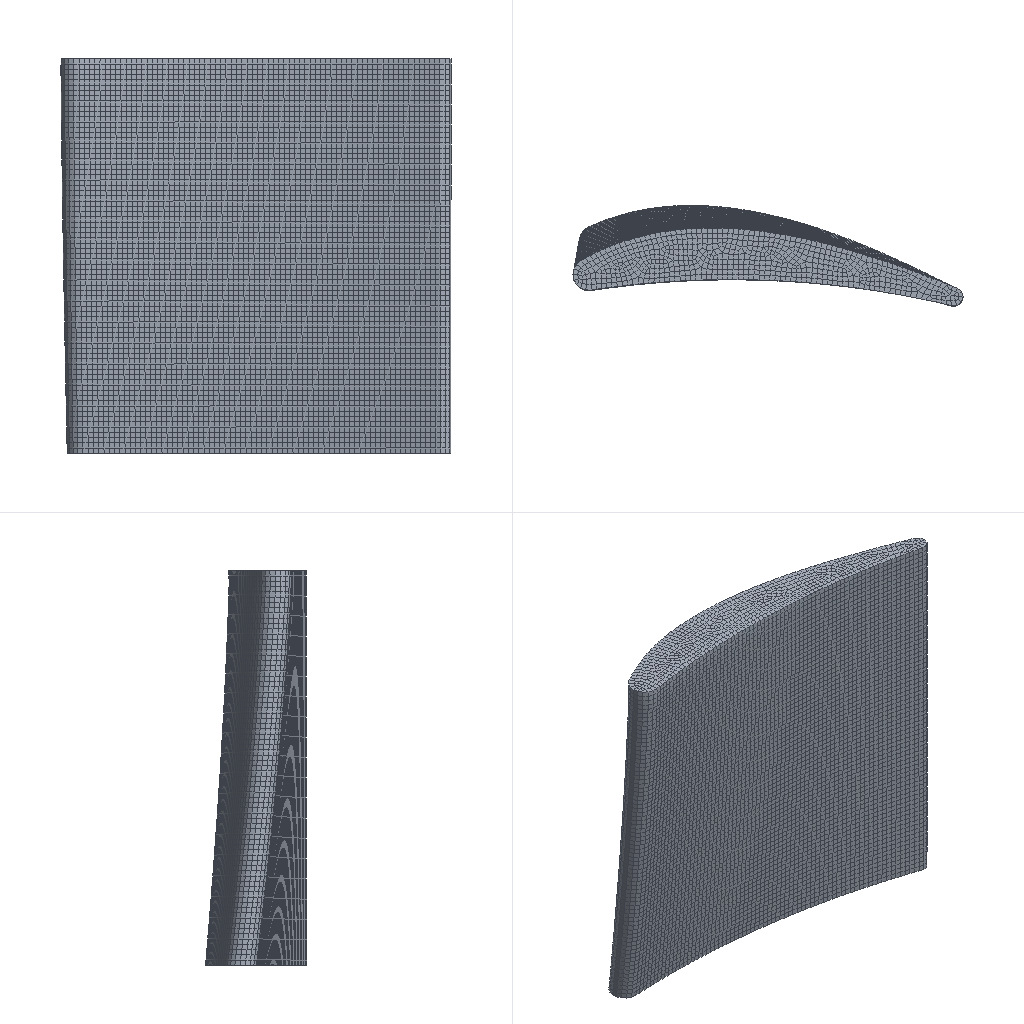Simulation study | abaqus
Set-up summary:
category,name,step,type,value,unit,region
solver,abaqus
solver,version,,,Abaqus/Explicit 2020
units,not stated in the deck,,not stated
analysis,deck,,transient,transient
load_step,Step-1,Step-1,transient
load_step,requested,,,1
mesh,nodes,,,58257
mesh,elements,,,54278
element_type,R3D3,,rigid,5378
element_type,C3D8R,,solid,48900
load,load commands in deck,,count,3
bc,support commands in deck,,count,7
material,MATERIAL-1,,in results
check,setup vs results,,match,"per instance, exact: element labels, types and connectivity; labels of the nodes the elements use; coordinates of those nodes at SINGLE_PRECISION in 2 of 2 instance(s)"
Abaqus input file, long lists of numbers shortened:
*Heading
** Job name: Job-1 Model name: Model-1
** Generated by: Abaqus/CAE 2020
*Preprint, echo=NO, model=NO, history=NO, contact=NO
**
** PARTS
**
*Part, name=tool-4
*Node
      1,           9.,           0.,         -90.
      2,          -9.,           0.,         -90.
** (2698 more lines like these left out)
*Element, type=R3D3
 1,   1, 149,   4
 2, 149, 178,   4
** (5376 more lines like these left out)
*Node
   2701,           0., -5.5109107e-16,         -90.
*Nset, nset=tool-4-RefPt_, internal
2701,
*Elset, elset=tool-4, generate
    1,  5378,     1
*End Part
**
*Part, name=work
*Node
      1,   43.691,  -25.705,         300.
      2,   39.949,  -24.243,         300.
** (55554 more lines like these left out)
*Element, type=C3D8R
    1,   667,   178,    32,   666,  1398,   909,   763,  1397
    2,   666,    32,    77,   431,  1397,   763,   808,  1162
** (48898 more lines like these left out)
*Nset, nset=Set-1, generate
     1,  55556,      1
*Elset, elset=Set-1, generate
     1,  48900,      1
** Section: Section-1
*Solid Section, elset=Set-1, material=Material-1
,
*End Part
**
**
** ASSEMBLY
**
*Assembly, name=Assembly
**
*Instance, name=tool-4-1, part=tool-4
  -45.177, 26.094, 89.811
  -45.177, 26.094, 89.811, -44.177, 26.094, 89.811, 5.
*End Instance
**
*Instance, name=work-1, part=work
   19.936,    15.042,        -100.
*End Instance
**
*Nset, nset=Set-1, instance=work-1, generate
   1,  731,    1
*Elset, elset=Set-1, instance=work-1, generate
   1,  652,    1
*Nset, nset=Set-2, instance=tool-4-1
 2701,
*Nset, nset=s_Set-3, instance=work-1, generate
     1,  55556,      1
*Elset, elset=s_Set-3, instance=work-1, generate
     1,  48900,      1
*Elset, elset=_m_Surf-1_SPOS, internal, instance=tool-4-1, generate
    1,  5378,     1
*Surface, type=ELEMENT, name=m_Surf-1
_m_Surf-1_SPOS, SPOS
*Surface, type=NODE, name=s_Set-3_CNS_, internal
s_Set-3, 1.
*Rigid Body, ref node=tool-4-1.tool-4-RefPt_, elset=tool-4-1.tool-4
*End Assembly
**
** MATERIALS
**
*Material, name=Material-1
*Damage Initiation, criterion=SHEAR
 0.1,0.,0.
*Damage Evolution, type=DISPLACEMENT
 1e-05,
*Density
 4.7e-09,
*Elastic
 1.2e+08, 0.28
*Plastic
800.,0.
**
** INTERACTION PROPERTIES
**
*Surface Interaction, name=IntProp-1
*Friction
 0.2,
*Surface Behavior, pressure-overclosure=HARD
** ----------------------------------------------------------------
**
** STEP: Step-1
**
*Step, name=Step-1, nlgeom=YES
*Dynamic, Explicit
, 0.08
*Bulk Viscosity
0.06, 1.2
** Mass Scaling: Semi-Automatic
**               Whole Model
*Fixed Mass Scaling, factor=5000.
**
** BOUNDARY CONDITIONS
**
** Name: BC-1 Type: 对称/反对称/完全固定
*Boundary
Set-1, ENCASTRE
** Name: [REDACTED] : Speed/Angular velocity
*Boundary, type=VELOCITY
Set-2, 1, 1, 2000.
Set-2, 2, 2, -2000.
Set-2, 3, 3
Set-2, 4, 4
Set-2, 5, 5
Set-2, 6, 6, 314.
**
** INTERACTIONS
**
** Interaction: Int-1
*Contact Pair, interaction=IntProp-1, mechanical constraint=KINEMATIC, cpset=Int-1
m_Surf-1, s_Set-3_CNS_
**
** OUTPUT REQUESTS
**
*Restart, write, number interval=1, time marks=NO
**
** FIELD OUTPUT: F-Output-1
**
*Output, field, number interval=50
*Node Output
A, CF, RF, RM, RT, U, V
*Element Output, directions=YES
E, EVF, LE, MISES, MISESMAX, PE, PEEQ, PEEQVAVG, PEVAVG, S, STATUS, SVAVG, YIELDPOT
*Contact Output
CSTRESS,
**
** HISTORY OUTPUT: H-Output-1
**
*Output, history, time interval=1.6e-06
*Node Output, nset=Set-2
RF1, RF2, RF3
*End Step
Results summary:
result,step,Step-1,partial,increments=47924 time=0.02234/0.08
result,analysis,,,transient
result,last_loadstep,,,1
result,primary field,,,U
result,reaction total,,FX,-37393.939,model units
result,reaction total,,FY,123420.848,model units
result,reaction total,,FZ,-35681.067,model units